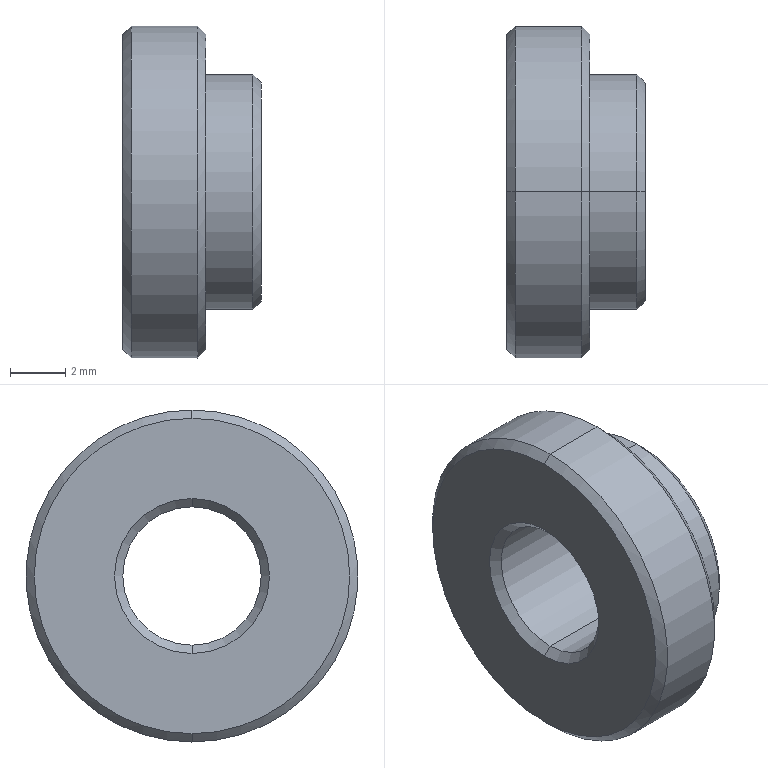Part | STEP file | ftcm_d8_5_h12_v5_0_t3_0_l5_0_2_03 | 1 solid | 19 faces | box 5 x 12 x 12 mm | volume 348.627 mm3 | cone 10 | cylinder 6 | plane 3 | commonest cylinder face diameters 5 x2 8.5 x2 12 x2
STEP:
#1=CARTESIAN_POINT('',(0.,0.,0.));
#2=DIRECTION('',(0.,0.,1.));
#3=DIRECTION('',(1.,0.,0.));
#4=AXIS2_PLACEMENT_3D('',#1,#2,#3);
#5=CARTESIAN_POINT('',(0.,0.,5.7));
#6=VERTEX_POINT('',#5);
#7=CARTESIAN_POINT('',(0.,0.,-5.7));
#8=VERTEX_POINT('',#7);
#9=CARTESIAN_POINT('',(0.,0.,0.));
#10=DIRECTION('',(-1.,0.,0.));
#11=DIRECTION('',(0.,0.,-1.));
#12=AXIS2_PLACEMENT_3D('',#9,#10,#11);
#13=CIRCLE('',#12,5.7);
#14=CARTESIAN_POINT('',(0.3,0.,0.));
#15=DIRECTION('',(1.,0.,0.));
#16=DIRECTION('',(0.,0.,-1.));
#17=AXIS2_PLACEMENT_3D('',#14,#15,#16);
#18=CONICAL_SURFACE('',#17,6.,0.7854);
#19=CARTESIAN_POINT('',(6.283,-0.3));
#20=DIRECTION('',(-1.,0.));
#21=VECTOR('',#20,1.);
#22=LINE('',#19,#21);
#23=(GEOMETRIC_REPRESENTATION_CONTEXT(2)PARAMETRIC_REPRESENTATION_CONTEXT()REPRESENTATION_CONTEXT('',''));
#24=DEFINITIONAL_REPRESENTATION('',(#22),#23);
#25=PCURVE('',#18,#24);
#26=CARTESIAN_POINT('',(0.,4.25,0.));
#27=DIRECTION('',(-1.,0.,0.));
#28=DIRECTION('',(0.,0.,1.));
#29=AXIS2_PLACEMENT_3D('',#26,#27,#28);
#30=PLANE('',#29);
#31=CARTESIAN_POINT('',(0.,-4.25));
#32=DIRECTION('',(-1.,0.));
#33=AXIS2_PLACEMENT_2D('',#31,#32);
#34=CIRCLE('',#33,5.7);
#35=(GEOMETRIC_REPRESENTATION_CONTEXT(2)PARAMETRIC_REPRESENTATION_CONTEXT()REPRESENTATION_CONTEXT('',''));
#36=DEFINITIONAL_REPRESENTATION('',(#34),#35);
#37=PCURVE('',#30,#36);
#38=SURFACE_CURVE('',#13,(#25,#37),.PCURVE_S1.);
#39=EDGE_CURVE('',#6,#8,#38,.T.);
#40=ORIENTED_EDGE('',*,*,#39,.F.);
#41=CARTESIAN_POINT('',(0.3,0.,6.));
#42=VERTEX_POINT('',#41);
#43=CARTESIAN_POINT('',(0.3,0.,6.));
#44=DIRECTION('',(0.7071,0.,0.7071));
#45=VECTOR('',#44,1.);
#46=LINE('',#43,#45);
#47=CARTESIAN_POINT('',(3.142,0.));
#48=DIRECTION('',(0.,1.));
#49=VECTOR('',#48,1.);
#50=LINE('',#47,#49);
#51=(GEOMETRIC_REPRESENTATION_CONTEXT(2)PARAMETRIC_REPRESENTATION_CONTEXT()REPRESENTATION_CONTEXT('',''));
#52=DEFINITIONAL_REPRESENTATION('',(#50),#51);
#53=PCURVE('',#18,#52);
#54=CARTESIAN_POINT('',(0.3,0.,0.));
#55=DIRECTION('',(1.,0.,0.));
#56=DIRECTION('',(0.,0.,-1.));
#57=AXIS2_PLACEMENT_3D('',#54,#55,#56);
#58=CONICAL_SURFACE('',#57,6.,0.7854);
#59=CARTESIAN_POINT('',(3.142,0.));
#60=DIRECTION('',(0.,1.));
#61=VECTOR('',#60,1.);
#62=LINE('',#59,#61);
#63=(GEOMETRIC_REPRESENTATION_CONTEXT(2)PARAMETRIC_REPRESENTATION_CONTEXT()REPRESENTATION_CONTEXT('',''));
#64=DEFINITIONAL_REPRESENTATION('',(#62),#63);
#65=PCURVE('',#58,#64);
#66=SURFACE_CURVE('',#46,(#53,#65),.PCURVE_S1.);
#67=EDGE_CURVE('',#6,#42,#66,.T.);
#68=ORIENTED_EDGE('',*,*,#67,.T.);
#69=CARTESIAN_POINT('',(0.3,0.,-6.));
#70=VERTEX_POINT('',#69);
#71=CARTESIAN_POINT('',(0.3,0.,0.));
#72=DIRECTION('',(-1.,0.,0.));
#73=DIRECTION('',(0.,1.,0.));
#74=AXIS2_PLACEMENT_3D('',#71,#72,#73);
#75=CIRCLE('',#74,6.);
#76=CARTESIAN_POINT('',(7.854,0.));
#77=DIRECTION('',(-1.,0.));
#78=VECTOR('',#77,1.);
#79=LINE('',#76,#78);
#80=(GEOMETRIC_REPRESENTATION_CONTEXT(2)PARAMETRIC_REPRESENTATION_CONTEXT()REPRESENTATION_CONTEXT('',''));
#81=DEFINITIONAL_REPRESENTATION('',(#79),#80);
#82=PCURVE('',#18,#81);
#83=CARTESIAN_POINT('',(1.5,0.,0.));
#84=DIRECTION('',(1.,0.,0.));
#85=DIRECTION('',(0.,0.,-1.));
#86=AXIS2_PLACEMENT_3D('',#83,#84,#85);
#87=CYLINDRICAL_SURFACE('',#86,6.);
#88=CARTESIAN_POINT('',(7.854,-1.2));
#89=DIRECTION('',(-1.,0.));
#90=VECTOR('',#89,1.);
#91=LINE('',#88,#90);
#92=(GEOMETRIC_REPRESENTATION_CONTEXT(2)PARAMETRIC_REPRESENTATION_CONTEXT()REPRESENTATION_CONTEXT('',''));
#93=DEFINITIONAL_REPRESENTATION('',(#91),#92);
#94=PCURVE('',#87,#93);
#95=SURFACE_CURVE('',#75,(#82,#94),.PCURVE_S1.);
#96=EDGE_CURVE('',#42,#70,#95,.T.);
#97=ORIENTED_EDGE('',*,*,#96,.T.);
#98=CARTESIAN_POINT('',(0.3,0.,-6.));
#99=DIRECTION('',(0.7071,0.,-0.7071));
#100=VECTOR('',#99,1.);
#101=LINE('',#98,#100);
#102=CARTESIAN_POINT('',(0.,0.));
#103=DIRECTION('',(0.,1.));
#104=VECTOR('',#103,1.);
#105=LINE('',#102,#104);
#106=(GEOMETRIC_REPRESENTATION_CONTEXT(2)PARAMETRIC_REPRESENTATION_CONTEXT()REPRESENTATION_CONTEXT('',''));
#107=DEFINITIONAL_REPRESENTATION('',(#105),#106);
#108=PCURVE('',#18,#107);
#109=CARTESIAN_POINT('',(6.283,0.));
#110=DIRECTION('',(0.,1.));
#111=VECTOR('',#110,1.);
#112=LINE('',#109,#111);
#113=(GEOMETRIC_REPRESENTATION_CONTEXT(2)PARAMETRIC_REPRESENTATION_CONTEXT()REPRESENTATION_CONTEXT('',''));
#114=DEFINITIONAL_REPRESENTATION('',(#112),#113);
#115=PCURVE('',#58,#114);
#116=SURFACE_CURVE('',#101,(#108,#115),.PCURVE_S1.);
#117=EDGE_CURVE('',#8,#70,#116,.T.);
#118=ORIENTED_EDGE('',*,*,#117,.F.);
#119=EDGE_LOOP('',(#40,#68,#97,#118));
#120=FACE_BOUND('',#119,.T.);
#121=ADVANCED_FACE('',(#120),#18,.T.);
#122=CARTESIAN_POINT('',(0.3,0.,2.5));
#123=VERTEX_POINT('',#122);
#124=CARTESIAN_POINT('',(0.,0.,2.8));
#125=VERTEX_POINT('',#124);
#126=CARTESIAN_POINT('',(0.,0.,2.8));
#127=DIRECTION('',(-0.7071,0.,0.7071));
#128=VECTOR('',#127,1.);
#129=LINE('',#126,#128);
#130=CARTESIAN_POINT('',(0.,0.,0.));
#131=DIRECTION('',(-1.,0.,0.));
#132=DIRECTION('',(0.,0.,1.));
#133=AXIS2_PLACEMENT_3D('',#130,#131,#132);
#134=CONICAL_SURFACE('',#133,2.8,0.7854);
#135=CARTESIAN_POINT('',(6.283,0.));
#136=DIRECTION('',(0.,1.));
#137=VECTOR('',#136,1.);
#138=LINE('',#135,#137);
#139=(GEOMETRIC_REPRESENTATION_CONTEXT(2)PARAMETRIC_REPRESENTATION_CONTEXT()REPRESENTATION_CONTEXT('',''));
#140=DEFINITIONAL_REPRESENTATION('',(#138),#139);
#141=PCURVE('',#134,#140);
#142=CARTESIAN_POINT('',(0.,0.,0.));
#143=DIRECTION('',(-1.,0.,0.));
#144=DIRECTION('',(0.,0.,1.));
#145=AXIS2_PLACEMENT_3D('',#142,#143,#144);
#146=CONICAL_SURFACE('',#145,2.8,0.7854);
#147=CARTESIAN_POINT('',(0.,0.));
#148=DIRECTION('',(0.,1.));
#149=VECTOR('',#148,1.);
#150=LINE('',#147,#149);
#151=(GEOMETRIC_REPRESENTATION_CONTEXT(2)PARAMETRIC_REPRESENTATION_CONTEXT()REPRESENTATION_CONTEXT('',''));
#152=DEFINITIONAL_REPRESENTATION('',(#150),#151);
#153=PCURVE('',#146,#152);
#154=SURFACE_CURVE('',#129,(#141,#153),.PCURVE_S1.);
#155=EDGE_CURVE('',#123,#125,#154,.T.);
#156=ORIENTED_EDGE('',*,*,#155,.T.);
#157=CARTESIAN_POINT('',(0.,0.,-2.8));
#158=VERTEX_POINT('',#157);
#159=CARTESIAN_POINT('',(0.,0.,0.));
#160=DIRECTION('',(1.,0.,0.));
#161=DIRECTION('',(0.,0.,1.));
#162=AXIS2_PLACEMENT_3D('',#159,#160,#161);
#163=CIRCLE('',#162,2.8);
#164=CARTESIAN_POINT('',(6.283,0.));
#165=DIRECTION('',(-1.,0.));
#166=VECTOR('',#165,1.);
#167=LINE('',#164,#166);
#168=(GEOMETRIC_REPRESENTATION_CONTEXT(2)PARAMETRIC_REPRESENTATION_CONTEXT()REPRESENTATION_CONTEXT('',''));
#169=DEFINITIONAL_REPRESENTATION('',(#167),#168);
#170=PCURVE('',#134,#169);
#171=CARTESIAN_POINT('',(2.8,-4.25));
#172=CARTESIAN_POINT('',(2.8,-9.1));
#173=CARTESIAN_POINT('',(-1.4,-6.675));
#174=CARTESIAN_POINT('',(-5.6,-4.25));
#175=CARTESIAN_POINT('',(-1.4,-1.825));
#176=CARTESIAN_POINT('',(2.8,0.5997));
#177=CARTESIAN_POINT('',(2.8,-4.25));
#178=(BOUNDED_CURVE()B_SPLINE_CURVE(2,(#171,#172,#173,#174,#175,#176,#177),.UNSPECIFIED.,.T.,.F.)B_SPLINE_CURVE_WITH_KNOTS((1,2,2,2,2,1),(-2.094,0.,2.094,4.189,6.283,8.378),.UNSPECIFIED.)CURVE()GEOMETRIC_REPRESENTATION_ITEM()RATIONAL_B_SPLINE_CURVE((1.,0.5,1.,0.5,1.,0.5,1.))REPRESENTATION_ITEM(''));
#179=(GEOMETRIC_REPRESENTATION_CONTEXT(2)PARAMETRIC_REPRESENTATION_CONTEXT()REPRESENTATION_CONTEXT('',''));
#180=DEFINITIONAL_REPRESENTATION('',(#178),#179);
#181=PCURVE('',#30,#180);
#182=SURFACE_CURVE('',#163,(#170,#181),.PCURVE_S1.);
#183=EDGE_CURVE('',#125,#158,#182,.T.);
#184=ORIENTED_EDGE('',*,*,#183,.T.);
#185=CARTESIAN_POINT('',(0.3,0.,-2.5));
#186=VERTEX_POINT('',#185);
#187=CARTESIAN_POINT('',(0.,0.,-2.8));
#188=DIRECTION('',(-0.7071,0.,-0.7071));
#189=VECTOR('',#188,1.);
#190=LINE('',#187,#189);
#191=CARTESIAN_POINT('',(3.142,0.));
#192=DIRECTION('',(0.,1.));
#193=VECTOR('',#192,1.);
#194=LINE('',#191,#193);
#195=(GEOMETRIC_REPRESENTATION_CONTEXT(2)PARAMETRIC_REPRESENTATION_CONTEXT()REPRESENTATION_CONTEXT('',''));
#196=DEFINITIONAL_REPRESENTATION('',(#194),#195);
#197=PCURVE('',#134,#196);
#198=CARTESIAN_POINT('',(3.142,0.));
#199=DIRECTION('',(0.,1.));
#200=VECTOR('',#199,1.);
#201=LINE('',#198,#200);
#202=(GEOMETRIC_REPRESENTATION_CONTEXT(2)PARAMETRIC_REPRESENTATION_CONTEXT()REPRESENTATION_CONTEXT('',''));
#203=DEFINITIONAL_REPRESENTATION('',(#201),#202);
#204=PCURVE('',#146,#203);
#205=SURFACE_CURVE('',#190,(#197,#204),.PCURVE_S1.);
#206=EDGE_CURVE('',#186,#158,#205,.T.);
#207=ORIENTED_EDGE('',*,*,#206,.F.);
#208=CARTESIAN_POINT('',(0.3,0.,0.));
#209=DIRECTION('',(-1.,0.,0.));
#210=DIRECTION('',(0.,1.,0.));
#211=AXIS2_PLACEMENT_3D('',#208,#209,#210);
#212=CIRCLE('',#211,2.5);
#213=CARTESIAN_POINT('',(1.571,-0.3));
#214=DIRECTION('',(1.,0.));
#215=VECTOR('',#214,1.);
#216=LINE('',#213,#215);
#217=(GEOMETRIC_REPRESENTATION_CONTEXT(2)PARAMETRIC_REPRESENTATION_CONTEXT()REPRESENTATION_CONTEXT('',''));
#218=DEFINITIONAL_REPRESENTATION('',(#216),#217);
#219=PCURVE('',#134,#218);
#220=CARTESIAN_POINT('',(2.5,0.,0.));
#221=DIRECTION('',(1.,0.,0.));
#222=DIRECTION('',(0.,0.,-1.));
#223=AXIS2_PLACEMENT_3D('',#220,#221,#222);
#224=CYLINDRICAL_SURFACE('',#223,2.5);
#225=CARTESIAN_POINT('',(7.854,-2.2));
#226=DIRECTION('',(-1.,0.));
#227=VECTOR('',#226,1.);
#228=LINE('',#225,#227);
#229=(GEOMETRIC_REPRESENTATION_CONTEXT(2)PARAMETRIC_REPRESENTATION_CONTEXT()REPRESENTATION_CONTEXT('',''));
#230=DEFINITIONAL_REPRESENTATION('',(#228),#229);
#231=PCURVE('',#224,#230);
#232=SURFACE_CURVE('',#212,(#219,#231),.PCURVE_S1.);
#233=EDGE_CURVE('',#186,#123,#232,.T.);
#234=ORIENTED_EDGE('',*,*,#233,.T.);
#235=EDGE_LOOP('',(#156,#184,#207,#234));
#236=FACE_BOUND('',#235,.F.);
#237=ADVANCED_FACE('',(#236),#134,.F.);
#238=ORIENTED_EDGE('',*,*,#96,.F.);
#239=CARTESIAN_POINT('',(2.7,0.,6.));
#240=VERTEX_POINT('',#239);
#241=CARTESIAN_POINT('',(1.5,0.,6.));
#242=DIRECTION('',(1.,0.,0.));
#243=VECTOR('',#242,1.);
#244=LINE('',#241,#243);
#245=CARTESIAN_POINT('',(3.142,0.));
#246=DIRECTION('',(0.,1.));
#247=VECTOR('',#246,1.);
#248=LINE('',#245,#247);
#249=(GEOMETRIC_REPRESENTATION_CONTEXT(2)PARAMETRIC_REPRESENTATION_CONTEXT()REPRESENTATION_CONTEXT('',''));
#250=DEFINITIONAL_REPRESENTATION('',(#248),#249);
#251=PCURVE('',#87,#250);
#252=CARTESIAN_POINT('',(1.5,0.,0.));
#253=DIRECTION('',(1.,0.,0.));
#254=DIRECTION('',(0.,0.,-1.));
#255=AXIS2_PLACEMENT_3D('',#252,#253,#254);
#256=CYLINDRICAL_SURFACE('',#255,6.);
#257=CARTESIAN_POINT('',(3.142,0.));
#258=DIRECTION('',(0.,1.));
#259=VECTOR('',#258,1.);
#260=LINE('',#257,#259);
#261=(GEOMETRIC_REPRESENTATION_CONTEXT(2)PARAMETRIC_REPRESENTATION_CONTEXT()REPRESENTATION_CONTEXT('',''));
#262=DEFINITIONAL_REPRESENTATION('',(#260),#261);
#263=PCURVE('',#256,#262);
#264=SURFACE_CURVE('',#244,(#251,#263),.PCURVE_S1.);
#265=EDGE_CURVE('',#42,#240,#264,.T.);
#266=ORIENTED_EDGE('',*,*,#265,.T.);
#267=CARTESIAN_POINT('',(2.7,0.,-6.));
#268=VERTEX_POINT('',#267);
#269=CARTESIAN_POINT('',(2.7,0.,0.));
#270=DIRECTION('',(-1.,0.,0.));
#271=DIRECTION('',(0.,0.,-1.));
#272=AXIS2_PLACEMENT_3D('',#269,#270,#271);
#273=CIRCLE('',#272,6.);
#274=CARTESIAN_POINT('',(6.283,1.2));
#275=DIRECTION('',(-1.,0.));
#276=VECTOR('',#275,1.);
#277=LINE('',#274,#276);
#278=(GEOMETRIC_REPRESENTATION_CONTEXT(2)PARAMETRIC_REPRESENTATION_CONTEXT()REPRESENTATION_CONTEXT('',''));
#279=DEFINITIONAL_REPRESENTATION('',(#277),#278);
#280=PCURVE('',#87,#279);
#281=CARTESIAN_POINT('',(2.7,0.,0.));
#282=DIRECTION('',(-1.,0.,0.));
#283=DIRECTION('',(0.,0.,1.));
#284=AXIS2_PLACEMENT_3D('',#281,#282,#283);
#285=CONICAL_SURFACE('',#284,6.,0.7854);
#286=CARTESIAN_POINT('',(-3.142,0.));
#287=DIRECTION('',(1.,0.));
#288=VECTOR('',#287,1.);
#289=LINE('',#286,#288);
#290=(GEOMETRIC_REPRESENTATION_CONTEXT(2)PARAMETRIC_REPRESENTATION_CONTEXT()REPRESENTATION_CONTEXT('',''));
#291=DEFINITIONAL_REPRESENTATION('',(#289),#290);
#292=PCURVE('',#285,#291);
#293=SURFACE_CURVE('',#273,(#280,#292),.PCURVE_S1.);
#294=EDGE_CURVE('',#240,#268,#293,.T.);
#295=ORIENTED_EDGE('',*,*,#294,.T.);
#296=CARTESIAN_POINT('',(1.5,0.,-6.));
#297=DIRECTION('',(1.,0.,0.));
#298=VECTOR('',#297,1.);
#299=LINE('',#296,#298);
#300=CARTESIAN_POINT('',(0.,0.));
#301=DIRECTION('',(0.,1.));
#302=VECTOR('',#301,1.);
#303=LINE('',#300,#302);
#304=(GEOMETRIC_REPRESENTATION_CONTEXT(2)PARAMETRIC_REPRESENTATION_CONTEXT()REPRESENTATION_CONTEXT('',''));
#305=DEFINITIONAL_REPRESENTATION('',(#303),#304);
#306=PCURVE('',#87,#305);
#307=CARTESIAN_POINT('',(6.283,0.));
#308=DIRECTION('',(0.,1.));
#309=VECTOR('',#308,1.);
#310=LINE('',#307,#309);
#311=(GEOMETRIC_REPRESENTATION_CONTEXT(2)PARAMETRIC_REPRESENTATION_CONTEXT()REPRESENTATION_CONTEXT('',''));
#312=DEFINITIONAL_REPRESENTATION('',(#310),#311);
#313=PCURVE('',#256,#312);
#314=SURFACE_CURVE('',#299,(#306,#313),.PCURVE_S1.);
#315=EDGE_CURVE('',#70,#268,#314,.T.);
#316=ORIENTED_EDGE('',*,*,#315,.F.);
#317=EDGE_LOOP('',(#238,#266,#295,#316));
#318=FACE_BOUND('',#317,.T.);
#319=ADVANCED_FACE('',(#318),#87,.T.);
#320=CARTESIAN_POINT('',(4.7,0.,-2.5));
#321=VERTEX_POINT('',#320);
#322=CARTESIAN_POINT('',(2.5,0.,-2.5));
#323=DIRECTION('',(1.,0.,0.));
#324=VECTOR('',#323,1.);
#325=LINE('',#322,#324);
#326=CARTESIAN_POINT('',(6.283,0.));
#327=DIRECTION('',(0.,1.));
#328=VECTOR('',#327,1.);
#329=LINE('',#326,#328);
#330=(GEOMETRIC_REPRESENTATION_CONTEXT(2)PARAMETRIC_REPRESENTATION_CONTEXT()REPRESENTATION_CONTEXT('',''));
#331=DEFINITIONAL_REPRESENTATION('',(#329),#330);
#332=PCURVE('',#224,#331);
#333=CARTESIAN_POINT('',(2.5,0.,0.));
#334=DIRECTION('',(1.,0.,0.));
#335=DIRECTION('',(0.,0.,-1.));
#336=AXIS2_PLACEMENT_3D('',#333,#334,#335);
#337=CYLINDRICAL_SURFACE('',#336,2.5);
#338=CARTESIAN_POINT('',(0.,0.));
#339=DIRECTION('',(0.,1.));
#340=VECTOR('',#339,1.);
#341=LINE('',#338,#340);
#342=(GEOMETRIC_REPRESENTATION_CONTEXT(2)PARAMETRIC_REPRESENTATION_CONTEXT()REPRESENTATION_CONTEXT('',''));
#343=DEFINITIONAL_REPRESENTATION('',(#341),#342);
#344=PCURVE('',#337,#343);
#345=SURFACE_CURVE('',#325,(#332,#344),.PCURVE_S1.);
#346=EDGE_CURVE('',#186,#321,#345,.T.);
#347=ORIENTED_EDGE('',*,*,#346,.T.);
#348=CARTESIAN_POINT('',(4.7,0.,2.5));
#349=VERTEX_POINT('',#348);
#350=CARTESIAN_POINT('',(4.7,0.,0.));
#351=DIRECTION('',(-1.,0.,0.));
#352=DIRECTION('',(0.,0.,-1.));
#353=AXIS2_PLACEMENT_3D('',#350,#351,#352);
#354=CIRCLE('',#353,2.5);
#355=CARTESIAN_POINT('',(6.283,2.2));
#356=DIRECTION('',(-1.,0.));
#357=VECTOR('',#356,1.);
#358=LINE('',#355,#357);
#359=(GEOMETRIC_REPRESENTATION_CONTEXT(2)PARAMETRIC_REPRESENTATION_CONTEXT()REPRESENTATION_CONTEXT('',''));
#360=DEFINITIONAL_REPRESENTATION('',(#358),#359);
#361=PCURVE('',#224,#360);
#362=CARTESIAN_POINT('',(5.,0.,0.));
#363=DIRECTION('',(1.,0.,0.));
#364=DIRECTION('',(0.,0.,-1.));
#365=AXIS2_PLACEMENT_3D('',#362,#363,#364);
#366=CONICAL_SURFACE('',#365,2.8,0.7854);
#367=CARTESIAN_POINT('',(6.283,-0.3));
#368=DIRECTION('',(-1.,0.));
#369=VECTOR('',#368,1.);
#370=LINE('',#367,#369);
#371=(GEOMETRIC_REPRESENTATION_CONTEXT(2)PARAMETRIC_REPRESENTATION_CONTEXT()REPRESENTATION_CONTEXT('',''));
#372=DEFINITIONAL_REPRESENTATION('',(#370),#371);
#373=PCURVE('',#366,#372);
#374=SURFACE_CURVE('',#354,(#361,#373),.PCURVE_S1.);
#375=EDGE_CURVE('',#321,#349,#374,.T.);
#376=ORIENTED_EDGE('',*,*,#375,.T.);
#377=CARTESIAN_POINT('',(2.5,0.,2.5));
#378=DIRECTION('',(1.,0.,0.));
#379=VECTOR('',#378,1.);
#380=LINE('',#377,#379);
#381=CARTESIAN_POINT('',(3.142,0.));
#382=DIRECTION('',(0.,1.));
#383=VECTOR('',#382,1.);
#384=LINE('',#381,#383);
#385=(GEOMETRIC_REPRESENTATION_CONTEXT(2)PARAMETRIC_REPRESENTATION_CONTEXT()REPRESENTATION_CONTEXT('',''));
#386=DEFINITIONAL_REPRESENTATION('',(#384),#385);
#387=PCURVE('',#224,#386);
#388=CARTESIAN_POINT('',(3.142,0.));
#389=DIRECTION('',(0.,1.));
#390=VECTOR('',#389,1.);
#391=LINE('',#388,#390);
#392=(GEOMETRIC_REPRESENTATION_CONTEXT(2)PARAMETRIC_REPRESENTATION_CONTEXT()REPRESENTATION_CONTEXT('',''));
#393=DEFINITIONAL_REPRESENTATION('',(#391),#392);
#394=PCURVE('',#337,#393);
#395=SURFACE_CURVE('',#380,(#387,#394),.PCURVE_S1.);
#396=EDGE_CURVE('',#123,#349,#395,.T.);
#397=ORIENTED_EDGE('',*,*,#396,.F.);
#398=ORIENTED_EDGE('',*,*,#233,.F.);
#399=EDGE_LOOP('',(#347,#376,#397,#398));
#400=FACE_BOUND('',#399,.F.);
#401=ADVANCED_FACE('',(#400),#224,.F.);
#402=CARTESIAN_POINT('',(3.,0.,5.7));
#403=VERTEX_POINT('',#402);
#404=CARTESIAN_POINT('',(3.,0.,-5.7));
#405=VERTEX_POINT('',#404);
#406=CARTESIAN_POINT('',(3.,0.,0.));
#407=DIRECTION('',(-1.,0.,0.));
#408=DIRECTION('',(0.,0.,1.));
#409=AXIS2_PLACEMENT_3D('',#406,#407,#408);
#410=CIRCLE('',#409,5.7);
#411=CARTESIAN_POINT('',(0.,-0.3));
#412=DIRECTION('',(1.,0.));
#413=VECTOR('',#412,1.);
#414=LINE('',#411,#413);
#415=(GEOMETRIC_REPRESENTATION_CONTEXT(2)PARAMETRIC_REPRESENTATION_CONTEXT()REPRESENTATION_CONTEXT('',''));
#416=DEFINITIONAL_REPRESENTATION('',(#414),#415);
#417=PCURVE('',#285,#416);
#418=CARTESIAN_POINT('',(3.,4.975,0.));
#419=DIRECTION('',(1.,0.,0.));
#420=DIRECTION('',(0.,0.,-1.));
#421=AXIS2_PLACEMENT_3D('',#418,#419,#420);
#422=PLANE('',#421);
#423=CARTESIAN_POINT('',(-5.7,-4.975));
#424=CARTESIAN_POINT('',(-5.7,4.898));
#425=CARTESIAN_POINT('',(2.85,-0.03866));
#426=CARTESIAN_POINT('',(11.4,-4.975));
#427=CARTESIAN_POINT('',(2.85,-9.911));
#428=CARTESIAN_POINT('',(-5.7,-14.848));
#429=CARTESIAN_POINT('',(-5.7,-4.975));
#430=(BOUNDED_CURVE()B_SPLINE_CURVE(2,(#423,#424,#425,#426,#427,#428,#429),.UNSPECIFIED.,.T.,.F.)B_SPLINE_CURVE_WITH_KNOTS((1,2,2,2,2,1),(-2.094,0.,2.094,4.189,6.283,8.378),.UNSPECIFIED.)CURVE()GEOMETRIC_REPRESENTATION_ITEM()RATIONAL_B_SPLINE_CURVE((1.,0.5,1.,0.5,1.,0.5,1.))REPRESENTATION_ITEM(''));
#431=(GEOMETRIC_REPRESENTATION_CONTEXT(2)PARAMETRIC_REPRESENTATION_CONTEXT()REPRESENTATION_CONTEXT('',''));
#432=DEFINITIONAL_REPRESENTATION('',(#430),#431);
#433=PCURVE('',#422,#432);
#434=SURFACE_CURVE('',#410,(#417,#433),.PCURVE_S1.);
#435=EDGE_CURVE('',#403,#405,#434,.T.);
#436=ORIENTED_EDGE('',*,*,#435,.T.);
#437=CARTESIAN_POINT('',(2.7,0.,-6.));
#438=DIRECTION('',(-0.7071,0.,-0.7071));
#439=VECTOR('',#438,1.);
#440=LINE('',#437,#439);
#441=CARTESIAN_POINT('',(3.142,0.));
#442=DIRECTION('',(0.,1.));
#443=VECTOR('',#442,1.);
#444=LINE('',#441,#443);
#445=(GEOMETRIC_REPRESENTATION_CONTEXT(2)PARAMETRIC_REPRESENTATION_CONTEXT()REPRESENTATION_CONTEXT('',''));
#446=DEFINITIONAL_REPRESENTATION('',(#444),#445);
#447=PCURVE('',#285,#446);
#448=CARTESIAN_POINT('',(2.7,0.,0.));
#449=DIRECTION('',(-1.,0.,0.));
#450=DIRECTION('',(0.,0.,1.));
#451=AXIS2_PLACEMENT_3D('',#448,#449,#450);
#452=CONICAL_SURFACE('',#451,6.,0.7854);
#453=CARTESIAN_POINT('',(3.142,0.));
#454=DIRECTION('',(0.,1.));
#455=VECTOR('',#454,1.);
#456=LINE('',#453,#455);
#457=(GEOMETRIC_REPRESENTATION_CONTEXT(2)PARAMETRIC_REPRESENTATION_CONTEXT()REPRESENTATION_CONTEXT('',''));
#458=DEFINITIONAL_REPRESENTATION('',(#456),#457);
#459=PCURVE('',#452,#458);
#460=SURFACE_CURVE('',#440,(#447,#459),.PCURVE_S1.);
#461=EDGE_CURVE('',#405,#268,#460,.T.);
#462=ORIENTED_EDGE('',*,*,#461,.T.);
#463=ORIENTED_EDGE('',*,*,#294,.F.);
#464=CARTESIAN_POINT('',(2.7,0.,6.));
#465=DIRECTION('',(-0.7071,0.,0.7071));
#466=VECTOR('',#465,1.);
#467=LINE('',#464,#466);
#468=CARTESIAN_POINT('',(0.,0.));
#469=DIRECTION('',(0.,1.));
#470=VECTOR('',#469,1.);
#471=LINE('',#468,#470);
#472=(GEOMETRIC_REPRESENTATION_CONTEXT(2)PARAMETRIC_REPRESENTATION_CONTEXT()REPRESENTATION_CONTEXT('',''));
#473=DEFINITIONAL_REPRESENTATION('',(#471),#472);
#474=PCURVE('',#285,#473);
#475=CARTESIAN_POINT('',(6.283,0.));
#476=DIRECTION('',(0.,1.));
#477=VECTOR('',#476,1.);
#478=LINE('',#475,#477);
#479=(GEOMETRIC_REPRESENTATION_CONTEXT(2)PARAMETRIC_REPRESENTATION_CONTEXT()REPRESENTATION_CONTEXT('',''));
#480=DEFINITIONAL_REPRESENTATION('',(#478),#479);
#481=PCURVE('',#452,#480);
#482=SURFACE_CURVE('',#467,(#474,#481),.PCURVE_S1.);
#483=EDGE_CURVE('',#403,#240,#482,.T.);
#484=ORIENTED_EDGE('',*,*,#483,.F.);
#485=EDGE_LOOP('',(#436,#462,#463,#484));
#486=FACE_BOUND('',#485,.T.);
#487=ADVANCED_FACE('',(#486),#285,.T.);
#488=CARTESIAN_POINT('',(5.,0.,-2.8));
#489=VERTEX_POINT('',#488);
#490=CARTESIAN_POINT('',(5.,0.,-2.8));
#491=DIRECTION('',(0.7071,0.,-0.7071));
#492=VECTOR('',#491,1.);
#493=LINE('',#490,#492);
#494=CARTESIAN_POINT('',(6.283,0.));
#495=DIRECTION('',(0.,1.));
#496=VECTOR('',#495,1.);
#497=LINE('',#494,#496);
#498=(GEOMETRIC_REPRESENTATION_CONTEXT(2)PARAMETRIC_REPRESENTATION_CONTEXT()REPRESENTATION_CONTEXT('',''));
#499=DEFINITIONAL_REPRESENTATION('',(#497),#498);
#500=PCURVE('',#366,#499);
#501=CARTESIAN_POINT('',(5.,0.,0.));
#502=DIRECTION('',(1.,0.,0.));
#503=DIRECTION('',(0.,0.,-1.));
#504=AXIS2_PLACEMENT_3D('',#501,#502,#503);
#505=CONICAL_SURFACE('',#504,2.8,0.7854);
#506=CARTESIAN_POINT('',(0.,0.));
#507=DIRECTION('',(0.,1.));
#508=VECTOR('',#507,1.);
#509=LINE('',#506,#508);
#510=(GEOMETRIC_REPRESENTATION_CONTEXT(2)PARAMETRIC_REPRESENTATION_CONTEXT()REPRESENTATION_CONTEXT('',''));
#511=DEFINITIONAL_REPRESENTATION('',(#509),#510);
#512=PCURVE('',#505,#511);
#513=SURFACE_CURVE('',#493,(#500,#512),.PCURVE_S1.);
#514=EDGE_CURVE('',#321,#489,#513,.T.);
#515=ORIENTED_EDGE('',*,*,#514,.T.);
#516=CARTESIAN_POINT('',(5.,0.,2.8));
#517=VERTEX_POINT('',#516);
#518=CARTESIAN_POINT('',(5.,0.,0.));
#519=DIRECTION('',(-1.,0.,0.));
#520=DIRECTION('',(0.,0.,-1.));
#521=AXIS2_PLACEMENT_3D('',#518,#519,#520);
#522=CIRCLE('',#521,2.8);
#523=CARTESIAN_POINT('',(6.283,0.));
#524=DIRECTION('',(-1.,0.));
#525=VECTOR('',#524,1.);
#526=LINE('',#523,#525);
#527=(GEOMETRIC_REPRESENTATION_CONTEXT(2)PARAMETRIC_REPRESENTATION_CONTEXT()REPRESENTATION_CONTEXT('',''));
#528=DEFINITIONAL_REPRESENTATION('',(#526),#527);
#529=PCURVE('',#366,#528);
#530=CARTESIAN_POINT('',(5.,3.375,0.));
#531=DIRECTION('',(1.,0.,0.));
#532=DIRECTION('',(0.,0.,-1.));
#533=AXIS2_PLACEMENT_3D('',#530,#531,#532);
#534=PLANE('',#533);
#535=CARTESIAN_POINT('',(2.8,-3.375));
#536=CARTESIAN_POINT('',(2.8,-8.225));
#537=CARTESIAN_POINT('',(-1.4,-5.8));
#538=CARTESIAN_POINT('',(-5.6,-3.375));
#539=CARTESIAN_POINT('',(-1.4,-0.9501));
#540=CARTESIAN_POINT('',(2.8,1.475));
#541=CARTESIAN_POINT('',(2.8,-3.375));
#542=(BOUNDED_CURVE()B_SPLINE_CURVE(2,(#535,#536,#537,#538,#539,#540,#541),.UNSPECIFIED.,.T.,.F.)B_SPLINE_CURVE_WITH_KNOTS((1,2,2,2,2,1),(-2.094,0.,2.094,4.189,6.283,8.378),.UNSPECIFIED.)CURVE()GEOMETRIC_REPRESENTATION_ITEM()RATIONAL_B_SPLINE_CURVE((1.,0.5,1.,0.5,1.,0.5,1.))REPRESENTATION_ITEM(''));
#543=(GEOMETRIC_REPRESENTATION_CONTEXT(2)PARAMETRIC_REPRESENTATION_CONTEXT()REPRESENTATION_CONTEXT('',''));
#544=DEFINITIONAL_REPRESENTATION('',(#542),#543);
#545=PCURVE('',#534,#544);
#546=SURFACE_CURVE('',#522,(#529,#545),.PCURVE_S1.);
#547=EDGE_CURVE('',#489,#517,#546,.T.);
#548=ORIENTED_EDGE('',*,*,#547,.T.);
#549=CARTESIAN_POINT('',(5.,0.,2.8));
#550=DIRECTION('',(0.7071,0.,0.7071));
#551=VECTOR('',#550,1.);
#552=LINE('',#549,#551);
#553=CARTESIAN_POINT('',(3.142,0.));
#554=DIRECTION('',(0.,1.));
#555=VECTOR('',#554,1.);
#556=LINE('',#553,#555);
#557=(GEOMETRIC_REPRESENTATION_CONTEXT(2)PARAMETRIC_REPRESENTATION_CONTEXT()REPRESENTATION_CONTEXT('',''));
#558=DEFINITIONAL_REPRESENTATION('',(#556),#557);
#559=PCURVE('',#366,#558);
#560=CARTESIAN_POINT('',(3.142,0.));
#561=DIRECTION('',(0.,1.));
#562=VECTOR('',#561,1.);
#563=LINE('',#560,#562);
#564=(GEOMETRIC_REPRESENTATION_CONTEXT(2)PARAMETRIC_REPRESENTATION_CONTEXT()REPRESENTATION_CONTEXT('',''));
#565=DEFINITIONAL_REPRESENTATION('',(#563),#564);
#566=PCURVE('',#505,#565);
#567=SURFACE_CURVE('',#552,(#559,#566),.PCURVE_S1.);
#568=EDGE_CURVE('',#349,#517,#567,.T.);
#569=ORIENTED_EDGE('',*,*,#568,.F.);
#570=ORIENTED_EDGE('',*,*,#375,.F.);
#571=EDGE_LOOP('',(#515,#548,#569,#570));
#572=FACE_BOUND('',#571,.F.);
#573=ADVANCED_FACE('',(#572),#366,.F.);
#574=CARTESIAN_POINT('',(3.,0.,4.25));
#575=VERTEX_POINT('',#574);
#576=CARTESIAN_POINT('',(3.,0.,-4.25));
#577=VERTEX_POINT('',#576);
#578=CARTESIAN_POINT('',(3.,0.,0.));
#579=DIRECTION('',(-1.,0.,0.));
#580=DIRECTION('',(0.,0.,-1.));
#581=AXIS2_PLACEMENT_3D('',#578,#579,#580);
#582=CIRCLE('',#581,4.25);
#583=CARTESIAN_POINT('',(3.85,0.,0.));
#584=DIRECTION('',(1.,0.,0.));
#585=DIRECTION('',(0.,0.,-1.));
#586=AXIS2_PLACEMENT_3D('',#583,#584,#585);
#587=CYLINDRICAL_SURFACE('',#586,4.25);
#588=CARTESIAN_POINT('',(6.283,-0.85));
#589=DIRECTION('',(-1.,0.));
#590=VECTOR('',#589,1.);
#591=LINE('',#588,#590);
#592=(GEOMETRIC_REPRESENTATION_CONTEXT(2)PARAMETRIC_REPRESENTATION_CONTEXT()REPRESENTATION_CONTEXT('',''));
#593=DEFINITIONAL_REPRESENTATION('',(#591),#592);
#594=PCURVE('',#587,#593);
#595=CARTESIAN_POINT('',(4.25,-4.975));
#596=CARTESIAN_POINT('',(4.25,-12.336));
#597=CARTESIAN_POINT('',(-2.125,-8.656));
#598=CARTESIAN_POINT('',(-8.5,-4.975));
#599=CARTESIAN_POINT('',(-2.125,-1.294));
#600=CARTESIAN_POINT('',(4.25,2.386));
#601=CARTESIAN_POINT('',(4.25,-4.975));
#602=(BOUNDED_CURVE()B_SPLINE_CURVE(2,(#595,#596,#597,#598,#599,#600,#601),.UNSPECIFIED.,.T.,.F.)B_SPLINE_CURVE_WITH_KNOTS((1,2,2,2,2,1),(-2.094,0.,2.094,4.189,6.283,8.378),.UNSPECIFIED.)CURVE()GEOMETRIC_REPRESENTATION_ITEM()RATIONAL_B_SPLINE_CURVE((1.,0.5,1.,0.5,1.,0.5,1.))REPRESENTATION_ITEM(''));
#603=(GEOMETRIC_REPRESENTATION_CONTEXT(2)PARAMETRIC_REPRESENTATION_CONTEXT()REPRESENTATION_CONTEXT('',''));
#604=DEFINITIONAL_REPRESENTATION('',(#602),#603);
#605=PCURVE('',#422,#604);
#606=SURFACE_CURVE('',#582,(#594,#605),.PCURVE_S1.);
#607=EDGE_CURVE('',#575,#577,#606,.T.);
#608=ORIENTED_EDGE('',*,*,#607,.F.);
#609=CARTESIAN_POINT('',(4.7,0.,4.25));
#610=VERTEX_POINT('',#609);
#611=CARTESIAN_POINT('',(3.85,0.,4.25));
#612=DIRECTION('',(1.,0.,0.));
#613=VECTOR('',#612,1.);
#614=LINE('',#611,#613);
#615=CARTESIAN_POINT('',(3.142,0.));
#616=DIRECTION('',(0.,1.));
#617=VECTOR('',#616,1.);
#618=LINE('',#615,#617);
#619=(GEOMETRIC_REPRESENTATION_CONTEXT(2)PARAMETRIC_REPRESENTATION_CONTEXT()REPRESENTATION_CONTEXT('',''));
#620=DEFINITIONAL_REPRESENTATION('',(#618),#619);
#621=PCURVE('',#587,#620);
#622=CARTESIAN_POINT('',(3.85,0.,0.));
#623=DIRECTION('',(1.,0.,0.));
#624=DIRECTION('',(0.,0.,-1.));
#625=AXIS2_PLACEMENT_3D('',#622,#623,#624);
#626=CYLINDRICAL_SURFACE('',#625,4.25);
#627=CARTESIAN_POINT('',(3.142,0.));
#628=DIRECTION('',(0.,1.));
#629=VECTOR('',#628,1.);
#630=LINE('',#627,#629);
#631=(GEOMETRIC_REPRESENTATION_CONTEXT(2)PARAMETRIC_REPRESENTATION_CONTEXT()REPRESENTATION_CONTEXT('',''));
#632=DEFINITIONAL_REPRESENTATION('',(#630),#631);
#633=PCURVE('',#626,#632);
#634=SURFACE_CURVE('',#614,(#621,#633),.PCURVE_S1.);
#635=EDGE_CURVE('',#575,#610,#634,.T.);
#636=ORIENTED_EDGE('',*,*,#635,.T.);
#637=CARTESIAN_POINT('',(4.7,0.,-4.25));
#638=VERTEX_POINT('',#637);
#639=CARTESIAN_POINT('',(4.7,0.,0.));
#640=DIRECTION('',(-1.,0.,0.));
#641=DIRECTION('',(0.,0.,-1.));
#642=AXIS2_PLACEMENT_3D('',#639,#640,#641);
#643=CIRCLE('',#642,4.25);
#644=CARTESIAN_POINT('',(6.283,0.85));
#645=DIRECTION('',(-1.,0.));
#646=VECTOR('',#645,1.);
#647=LINE('',#644,#646);
#648=(GEOMETRIC_REPRESENTATION_CONTEXT(2)PARAMETRIC_REPRESENTATION_CONTEXT()REPRESENTATION_CONTEXT('',''));
#649=DEFINITIONAL_REPRESENTATION('',(#647),#648);
#650=PCURVE('',#587,#649);
#651=CARTESIAN_POINT('',(4.7,0.,0.));
#652=DIRECTION('',(-1.,0.,0.));
#653=DIRECTION('',(0.,0.,1.));
#654=AXIS2_PLACEMENT_3D('',#651,#652,#653);
#655=CONICAL_SURFACE('',#654,4.25,0.7854);
#656=CARTESIAN_POINT('',(-3.142,0.));
#657=DIRECTION('',(1.,0.));
#658=VECTOR('',#657,1.);
#659=LINE('',#656,#658);
#660=(GEOMETRIC_REPRESENTATION_CONTEXT(2)PARAMETRIC_REPRESENTATION_CONTEXT()REPRESENTATION_CONTEXT('',''));
#661=DEFINITIONAL_REPRESENTATION('',(#659),#660);
#662=PCURVE('',#655,#661);
#663=SURFACE_CURVE('',#643,(#650,#662),.PCURVE_S1.);
#664=EDGE_CURVE('',#610,#638,#663,.T.);
#665=ORIENTED_EDGE('',*,*,#664,.T.);
#666=CARTESIAN_POINT('',(3.85,0.,-4.25));
#667=DIRECTION('',(1.,0.,0.));
#668=VECTOR('',#667,1.);
#669=LINE('',#666,#668);
#670=CARTESIAN_POINT('',(0.,0.));
#671=DIRECTION('',(0.,1.));
#672=VECTOR('',#671,1.);
#673=LINE('',#670,#672);
#674=(GEOMETRIC_REPRESENTATION_CONTEXT(2)PARAMETRIC_REPRESENTATION_CONTEXT()REPRESENTATION_CONTEXT('',''));
#675=DEFINITIONAL_REPRESENTATION('',(#673),#674);
#676=PCURVE('',#587,#675);
#677=CARTESIAN_POINT('',(6.283,0.));
#678=DIRECTION('',(0.,1.));
#679=VECTOR('',#678,1.);
#680=LINE('',#677,#679);
#681=(GEOMETRIC_REPRESENTATION_CONTEXT(2)PARAMETRIC_REPRESENTATION_CONTEXT()REPRESENTATION_CONTEXT('',''));
#682=DEFINITIONAL_REPRESENTATION('',(#680),#681);
#683=PCURVE('',#626,#682);
#684=SURFACE_CURVE('',#669,(#676,#683),.PCURVE_S1.);
#685=EDGE_CURVE('',#577,#638,#684,.T.);
#686=ORIENTED_EDGE('',*,*,#685,.F.);
#687=EDGE_LOOP('',(#608,#636,#665,#686));
#688=FACE_BOUND('',#687,.T.);
#689=ADVANCED_FACE('',(#688),#587,.T.);
#690=CARTESIAN_POINT('',(5.,0.,-3.95));
#691=VERTEX_POINT('',#690);
#692=CARTESIAN_POINT('',(5.,0.,3.95));
#693=VERTEX_POINT('',#692);
#694=CARTESIAN_POINT('',(5.,0.,0.));
#695=DIRECTION('',(1.,0.,0.));
#696=DIRECTION('',(0.,0.,1.));
#697=AXIS2_PLACEMENT_3D('',#694,#695,#696);
#698=CIRCLE('',#697,3.95);
#699=CARTESIAN_POINT('',(6.283,-0.3));
#700=DIRECTION('',(-1.,0.));
#701=VECTOR('',#700,1.);
#702=LINE('',#699,#701);
#703=(GEOMETRIC_REPRESENTATION_CONTEXT(2)PARAMETRIC_REPRESENTATION_CONTEXT()REPRESENTATION_CONTEXT('',''));
#704=DEFINITIONAL_REPRESENTATION('',(#702),#703);
#705=PCURVE('',#655,#704);
#706=CARTESIAN_POINT('',(0.,-3.375));
#707=DIRECTION('',(-1.,0.));
#708=AXIS2_PLACEMENT_2D('',#706,#707);
#709=CIRCLE('',#708,3.95);
#710=(GEOMETRIC_REPRESENTATION_CONTEXT(2)PARAMETRIC_REPRESENTATION_CONTEXT()REPRESENTATION_CONTEXT('',''));
#711=DEFINITIONAL_REPRESENTATION('',(#709),#710);
#712=PCURVE('',#534,#711);
#713=SURFACE_CURVE('',#698,(#705,#712),.PCURVE_S1.);
#714=EDGE_CURVE('',#691,#693,#713,.T.);
#715=ORIENTED_EDGE('',*,*,#714,.F.);
#716=CARTESIAN_POINT('',(4.7,0.,-4.25));
#717=DIRECTION('',(-0.7071,0.,-0.7071));
#718=VECTOR('',#717,1.);
#719=LINE('',#716,#718);
#720=CARTESIAN_POINT('',(3.142,0.));
#721=DIRECTION('',(0.,1.));
#722=VECTOR('',#721,1.);
#723=LINE('',#720,#722);
#724=(GEOMETRIC_REPRESENTATION_CONTEXT(2)PARAMETRIC_REPRESENTATION_CONTEXT()REPRESENTATION_CONTEXT('',''));
#725=DEFINITIONAL_REPRESENTATION('',(#723),#724);
#726=PCURVE('',#655,#725);
#727=CARTESIAN_POINT('',(4.7,0.,0.));
#728=DIRECTION('',(-1.,0.,0.));
#729=DIRECTION('',(0.,0.,1.));
#730=AXIS2_PLACEMENT_3D('',#727,#728,#729);
#731=CONICAL_SURFACE('',#730,4.25,0.7854);
#732=CARTESIAN_POINT('',(3.142,0.));
#733=DIRECTION('',(0.,1.));
#734=VECTOR('',#733,1.);
#735=LINE('',#732,#734);
#736=(GEOMETRIC_REPRESENTATION_CONTEXT(2)PARAMETRIC_REPRESENTATION_CONTEXT()REPRESENTATION_CONTEXT('',''));
#737=DEFINITIONAL_REPRESENTATION('',(#735),#736);
#738=PCURVE('',#731,#737);
#739=SURFACE_CURVE('',#719,(#726,#738),.PCURVE_S1.);
#740=EDGE_CURVE('',#691,#638,#739,.T.);
#741=ORIENTED_EDGE('',*,*,#740,.T.);
#742=ORIENTED_EDGE('',*,*,#664,.F.);
#743=CARTESIAN_POINT('',(4.7,0.,4.25));
#744=DIRECTION('',(-0.7071,0.,0.7071));
#745=VECTOR('',#744,1.);
#746=LINE('',#743,#745);
#747=CARTESIAN_POINT('',(0.,0.));
#748=DIRECTION('',(0.,1.));
#749=VECTOR('',#748,1.);
#750=LINE('',#747,#749);
#751=(GEOMETRIC_REPRESENTATION_CONTEXT(2)PARAMETRIC_REPRESENTATION_CONTEXT()REPRESENTATION_CONTEXT('',''));
#752=DEFINITIONAL_REPRESENTATION('',(#750),#751);
#753=PCURVE('',#655,#752);
#754=CARTESIAN_POINT('',(6.283,0.));
#755=DIRECTION('',(0.,1.));
#756=VECTOR('',#755,1.);
#757=LINE('',#754,#756);
#758=(GEOMETRIC_REPRESENTATION_CONTEXT(2)PARAMETRIC_REPRESENTATION_CONTEXT()REPRESENTATION_CONTEXT('',''));
#759=DEFINITIONAL_REPRESENTATION('',(#757),#758);
#760=PCURVE('',#731,#759);
#761=SURFACE_CURVE('',#746,(#753,#760),.PCURVE_S1.);
#762=EDGE_CURVE('',#693,#610,#761,.T.);
#763=ORIENTED_EDGE('',*,*,#762,.F.);
#764=EDGE_LOOP('',(#715,#741,#742,#763));
#765=FACE_BOUND('',#764,.T.);
#766=ADVANCED_FACE('',(#765),#655,.T.);
#767=CARTESIAN_POINT('',(0.,0.,0.));
#768=DIRECTION('',(-1.,0.,0.));
#769=DIRECTION('',(0.,0.,-1.));
#770=AXIS2_PLACEMENT_3D('',#767,#768,#769);
#771=CIRCLE('',#770,5.7);
#772=CARTESIAN_POINT('',(0.,-4.25));
#773=DIRECTION('',(-1.,0.));
#774=AXIS2_PLACEMENT_2D('',#772,#773);
#775=CIRCLE('',#774,5.7);
#776=(GEOMETRIC_REPRESENTATION_CONTEXT(2)PARAMETRIC_REPRESENTATION_CONTEXT()REPRESENTATION_CONTEXT('',''));
#777=DEFINITIONAL_REPRESENTATION('',(#775),#776);
#778=PCURVE('',#30,#777);
#779=CARTESIAN_POINT('',(6.283,-0.3));
#780=DIRECTION('',(-1.,0.));
#781=VECTOR('',#780,1.);
#782=LINE('',#779,#781);
#783=(GEOMETRIC_REPRESENTATION_CONTEXT(2)PARAMETRIC_REPRESENTATION_CONTEXT()REPRESENTATION_CONTEXT('',''));
#784=DEFINITIONAL_REPRESENTATION('',(#782),#783);
#785=PCURVE('',#58,#784);
#786=SURFACE_CURVE('',#771,(#778,#785),.PCURVE_S1.);
#787=EDGE_CURVE('',#8,#6,#786,.T.);
#788=ORIENTED_EDGE('',*,*,#787,.T.);
#789=ORIENTED_EDGE('',*,*,#39,.T.);
#790=EDGE_LOOP('',(#788,#789));
#791=FACE_BOUND('',#790,.T.);
#792=ORIENTED_EDGE('',*,*,#183,.T.);
#793=CARTESIAN_POINT('',(0.,0.,0.));
#794=DIRECTION('',(1.,0.,0.));
#795=DIRECTION('',(0.,0.,1.));
#796=AXIS2_PLACEMENT_3D('',#793,#794,#795);
#797=CIRCLE('',#796,2.8);
#798=CARTESIAN_POINT('',(2.8,-4.25));
#799=CARTESIAN_POINT('',(2.8,-9.1));
#800=CARTESIAN_POINT('',(-1.4,-6.675));
#801=CARTESIAN_POINT('',(-5.6,-4.25));
#802=CARTESIAN_POINT('',(-1.4,-1.825));
#803=CARTESIAN_POINT('',(2.8,0.5997));
#804=CARTESIAN_POINT('',(2.8,-4.25));
#805=(BOUNDED_CURVE()B_SPLINE_CURVE(2,(#798,#799,#800,#801,#802,#803,#804),.UNSPECIFIED.,.T.,.F.)B_SPLINE_CURVE_WITH_KNOTS((1,2,2,2,2,1),(-2.094,0.,2.094,4.189,6.283,8.378),.UNSPECIFIED.)CURVE()GEOMETRIC_REPRESENTATION_ITEM()RATIONAL_B_SPLINE_CURVE((1.,0.5,1.,0.5,1.,0.5,1.))REPRESENTATION_ITEM(''));
#806=(GEOMETRIC_REPRESENTATION_CONTEXT(2)PARAMETRIC_REPRESENTATION_CONTEXT()REPRESENTATION_CONTEXT('',''));
#807=DEFINITIONAL_REPRESENTATION('',(#805),#806);
#808=PCURVE('',#30,#807);
#809=CARTESIAN_POINT('',(6.283,0.));
#810=DIRECTION('',(-1.,0.));
#811=VECTOR('',#810,1.);
#812=LINE('',#809,#811);
#813=(GEOMETRIC_REPRESENTATION_CONTEXT(2)PARAMETRIC_REPRESENTATION_CONTEXT()REPRESENTATION_CONTEXT('',''));
#814=DEFINITIONAL_REPRESENTATION('',(#812),#813);
#815=PCURVE('',#146,#814);
#816=SURFACE_CURVE('',#797,(#808,#815),.PCURVE_S1.);
#817=EDGE_CURVE('',#158,#125,#816,.T.);
#818=ORIENTED_EDGE('',*,*,#817,.T.);
#819=EDGE_LOOP('',(#792,#818));
#820=FACE_BOUND('',#819,.T.);
#821=ADVANCED_FACE('',(#791,#820),#30,.T.);
#822=ORIENTED_EDGE('',*,*,#67,.F.);
#823=ORIENTED_EDGE('',*,*,#787,.F.);
#824=ORIENTED_EDGE('',*,*,#117,.T.);
#825=CARTESIAN_POINT('',(0.3,0.,0.));
#826=DIRECTION('',(-1.,0.,0.));
#827=DIRECTION('',(0.,1.,0.));
#828=AXIS2_PLACEMENT_3D('',#825,#826,#827);
#829=CIRCLE('',#828,6.);
#830=CARTESIAN_POINT('',(7.854,0.));
#831=DIRECTION('',(-1.,0.));
#832=VECTOR('',#831,1.);
#833=LINE('',#830,#832);
#834=(GEOMETRIC_REPRESENTATION_CONTEXT(2)PARAMETRIC_REPRESENTATION_CONTEXT()REPRESENTATION_CONTEXT('',''));
#835=DEFINITIONAL_REPRESENTATION('',(#833),#834);
#836=PCURVE('',#58,#835);
#837=CARTESIAN_POINT('',(7.854,-1.2));
#838=DIRECTION('',(-1.,0.));
#839=VECTOR('',#838,1.);
#840=LINE('',#837,#839);
#841=(GEOMETRIC_REPRESENTATION_CONTEXT(2)PARAMETRIC_REPRESENTATION_CONTEXT()REPRESENTATION_CONTEXT('',''));
#842=DEFINITIONAL_REPRESENTATION('',(#840),#841);
#843=PCURVE('',#256,#842);
#844=SURFACE_CURVE('',#829,(#836,#843),.PCURVE_S1.);
#845=EDGE_CURVE('',#70,#42,#844,.T.);
#846=ORIENTED_EDGE('',*,*,#845,.T.);
#847=EDGE_LOOP('',(#822,#823,#824,#846));
#848=FACE_BOUND('',#847,.T.);
#849=ADVANCED_FACE('',(#848),#58,.T.);
#850=ORIENTED_EDGE('',*,*,#817,.T.);
#851=ORIENTED_EDGE('',*,*,#155,.F.);
#852=CARTESIAN_POINT('',(0.3,0.,0.));
#853=DIRECTION('',(-1.,0.,0.));
#854=DIRECTION('',(0.,1.,0.));
#855=AXIS2_PLACEMENT_3D('',#852,#853,#854);
#856=CIRCLE('',#855,2.5);
#857=CARTESIAN_POINT('',(-4.712,-0.3));
#858=DIRECTION('',(1.,0.));
#859=VECTOR('',#858,1.);
#860=LINE('',#857,#859);
#861=(GEOMETRIC_REPRESENTATION_CONTEXT(2)PARAMETRIC_REPRESENTATION_CONTEXT()REPRESENTATION_CONTEXT('',''));
#862=DEFINITIONAL_REPRESENTATION('',(#860),#861);
#863=PCURVE('',#146,#862);
#864=CARTESIAN_POINT('',(7.854,-2.2));
#865=DIRECTION('',(-1.,0.));
#866=VECTOR('',#865,1.);
#867=LINE('',#864,#866);
#868=(GEOMETRIC_REPRESENTATION_CONTEXT(2)PARAMETRIC_REPRESENTATION_CONTEXT()REPRESENTATION_CONTEXT('',''));
#869=DEFINITIONAL_REPRESENTATION('',(#867),#868);
#870=PCURVE('',#337,#869);
#871=SURFACE_CURVE('',#856,(#863,#870),.PCURVE_S1.);
#872=EDGE_CURVE('',#123,#186,#871,.T.);
#873=ORIENTED_EDGE('',*,*,#872,.T.);
#874=ORIENTED_EDGE('',*,*,#206,.T.);
#875=EDGE_LOOP('',(#850,#851,#873,#874));
#876=FACE_BOUND('',#875,.F.);
#877=ADVANCED_FACE('',(#876),#146,.F.);
#878=ORIENTED_EDGE('',*,*,#265,.F.);
#879=ORIENTED_EDGE('',*,*,#845,.F.);
#880=ORIENTED_EDGE('',*,*,#315,.T.);
#881=CARTESIAN_POINT('',(2.7,0.,0.));
#882=DIRECTION('',(-1.,0.,0.));
#883=DIRECTION('',(0.,0.,-1.));
#884=AXIS2_PLACEMENT_3D('',#881,#882,#883);
#885=CIRCLE('',#884,6.);
#886=CARTESIAN_POINT('',(6.283,1.2));
#887=DIRECTION('',(-1.,0.));
#888=VECTOR('',#887,1.);
#889=LINE('',#886,#888);
#890=(GEOMETRIC_REPRESENTATION_CONTEXT(2)PARAMETRIC_REPRESENTATION_CONTEXT()REPRESENTATION_CONTEXT('',''));
#891=DEFINITIONAL_REPRESENTATION('',(#889),#890);
#892=PCURVE('',#256,#891);
#893=CARTESIAN_POINT('',(3.142,0.));
#894=DIRECTION('',(1.,0.));
#895=VECTOR('',#894,1.);
#896=LINE('',#893,#895);
#897=(GEOMETRIC_REPRESENTATION_CONTEXT(2)PARAMETRIC_REPRESENTATION_CONTEXT()REPRESENTATION_CONTEXT('',''));
#898=DEFINITIONAL_REPRESENTATION('',(#896),#897);
#899=PCURVE('',#452,#898);
#900=SURFACE_CURVE('',#885,(#892,#899),.PCURVE_S1.);
#901=EDGE_CURVE('',#268,#240,#900,.T.);
#902=ORIENTED_EDGE('',*,*,#901,.T.);
#903=EDGE_LOOP('',(#878,#879,#880,#902));
#904=FACE_BOUND('',#903,.T.);
#905=ADVANCED_FACE('',(#904),#256,.T.);
#906=CARTESIAN_POINT('',(4.7,0.,0.));
#907=DIRECTION('',(-1.,0.,0.));
#908=DIRECTION('',(0.,0.,-1.));
#909=AXIS2_PLACEMENT_3D('',#906,#907,#908);
#910=CIRCLE('',#909,2.5);
#911=CARTESIAN_POINT('',(6.283,2.2));
#912=DIRECTION('',(-1.,0.));
#913=VECTOR('',#912,1.);
#914=LINE('',#911,#913);
#915=(GEOMETRIC_REPRESENTATION_CONTEXT(2)PARAMETRIC_REPRESENTATION_CONTEXT()REPRESENTATION_CONTEXT('',''));
#916=DEFINITIONAL_REPRESENTATION('',(#914),#915);
#917=PCURVE('',#337,#916);
#918=CARTESIAN_POINT('',(6.283,-0.3));
#919=DIRECTION('',(-1.,0.));
#920=VECTOR('',#919,1.);
#921=LINE('',#918,#920);
#922=(GEOMETRIC_REPRESENTATION_CONTEXT(2)PARAMETRIC_REPRESENTATION_CONTEXT()REPRESENTATION_CONTEXT('',''));
#923=DEFINITIONAL_REPRESENTATION('',(#921),#922);
#924=PCURVE('',#505,#923);
#925=SURFACE_CURVE('',#910,(#917,#924),.PCURVE_S1.);
#926=EDGE_CURVE('',#349,#321,#925,.T.);
#927=ORIENTED_EDGE('',*,*,#926,.T.);
#928=ORIENTED_EDGE('',*,*,#346,.F.);
#929=ORIENTED_EDGE('',*,*,#872,.F.);
#930=ORIENTED_EDGE('',*,*,#396,.T.);
#931=EDGE_LOOP('',(#927,#928,#929,#930));
#932=FACE_BOUND('',#931,.F.);
#933=ADVANCED_FACE('',(#932),#337,.F.);
#934=ORIENTED_EDGE('',*,*,#461,.F.);
#935=CARTESIAN_POINT('',(3.,0.,0.));
#936=DIRECTION('',(-1.,0.,0.));
#937=DIRECTION('',(0.,0.,1.));
#938=AXIS2_PLACEMENT_3D('',#935,#936,#937);
#939=CIRCLE('',#938,5.7);
#940=CARTESIAN_POINT('',(0.,-0.3));
#941=DIRECTION('',(1.,0.));
#942=VECTOR('',#941,1.);
#943=LINE('',#940,#942);
#944=(GEOMETRIC_REPRESENTATION_CONTEXT(2)PARAMETRIC_REPRESENTATION_CONTEXT()REPRESENTATION_CONTEXT('',''));
#945=DEFINITIONAL_REPRESENTATION('',(#943),#944);
#946=PCURVE('',#452,#945);
#947=CARTESIAN_POINT('',(-5.7,-4.975));
#948=CARTESIAN_POINT('',(-5.7,4.898));
#949=CARTESIAN_POINT('',(2.85,-0.03866));
#950=CARTESIAN_POINT('',(11.4,-4.975));
#951=CARTESIAN_POINT('',(2.85,-9.911));
#952=CARTESIAN_POINT('',(-5.7,-14.848));
#953=CARTESIAN_POINT('',(-5.7,-4.975));
#954=(BOUNDED_CURVE()B_SPLINE_CURVE(2,(#947,#948,#949,#950,#951,#952,#953),.UNSPECIFIED.,.T.,.F.)B_SPLINE_CURVE_WITH_KNOTS((1,2,2,2,2,1),(-2.094,0.,2.094,4.189,6.283,8.378),.UNSPECIFIED.)CURVE()GEOMETRIC_REPRESENTATION_ITEM()RATIONAL_B_SPLINE_CURVE((1.,0.5,1.,0.5,1.,0.5,1.))REPRESENTATION_ITEM(''));
#955=(GEOMETRIC_REPRESENTATION_CONTEXT(2)PARAMETRIC_REPRESENTATION_CONTEXT()REPRESENTATION_CONTEXT('',''));
#956=DEFINITIONAL_REPRESENTATION('',(#954),#955);
#957=PCURVE('',#422,#956);
#958=SURFACE_CURVE('',#939,(#946,#957),.PCURVE_S1.);
#959=EDGE_CURVE('',#405,#403,#958,.T.);
#960=ORIENTED_EDGE('',*,*,#959,.T.);
#961=ORIENTED_EDGE('',*,*,#483,.T.);
#962=ORIENTED_EDGE('',*,*,#901,.F.);
#963=EDGE_LOOP('',(#934,#960,#961,#962));
#964=FACE_BOUND('',#963,.T.);
#965=ADVANCED_FACE('',(#964),#452,.T.);
#966=CARTESIAN_POINT('',(5.,0.,0.));
#967=DIRECTION('',(-1.,0.,0.));
#968=DIRECTION('',(0.,0.,-1.));
#969=AXIS2_PLACEMENT_3D('',#966,#967,#968);
#970=CIRCLE('',#969,2.8);
#971=CARTESIAN_POINT('',(6.283,0.));
#972=DIRECTION('',(-1.,0.));
#973=VECTOR('',#972,1.);
#974=LINE('',#971,#973);
#975=(GEOMETRIC_REPRESENTATION_CONTEXT(2)PARAMETRIC_REPRESENTATION_CONTEXT()REPRESENTATION_CONTEXT('',''));
#976=DEFINITIONAL_REPRESENTATION('',(#974),#975);
#977=PCURVE('',#505,#976);
#978=CARTESIAN_POINT('',(2.8,-3.375));
#979=CARTESIAN_POINT('',(2.8,-8.225));
#980=CARTESIAN_POINT('',(-1.4,-5.8));
#981=CARTESIAN_POINT('',(-5.6,-3.375));
#982=CARTESIAN_POINT('',(-1.4,-0.9501));
#983=CARTESIAN_POINT('',(2.8,1.475));
#984=CARTESIAN_POINT('',(2.8,-3.375));
#985=(BOUNDED_CURVE()B_SPLINE_CURVE(2,(#978,#979,#980,#981,#982,#983,#984),.UNSPECIFIED.,.T.,.F.)B_SPLINE_CURVE_WITH_KNOTS((1,2,2,2,2,1),(-2.094,0.,2.094,4.189,6.283,8.378),.UNSPECIFIED.)CURVE()GEOMETRIC_REPRESENTATION_ITEM()RATIONAL_B_SPLINE_CURVE((1.,0.5,1.,0.5,1.,0.5,1.))REPRESENTATION_ITEM(''));
#986=(GEOMETRIC_REPRESENTATION_CONTEXT(2)PARAMETRIC_REPRESENTATION_CONTEXT()REPRESENTATION_CONTEXT('',''));
#987=DEFINITIONAL_REPRESENTATION('',(#985),#986);
#988=PCURVE('',#534,#987);
#989=SURFACE_CURVE('',#970,(#977,#988),.PCURVE_S1.);
#990=EDGE_CURVE('',#517,#489,#989,.T.);
#991=ORIENTED_EDGE('',*,*,#990,.T.);
#992=ORIENTED_EDGE('',*,*,#514,.F.);
#993=ORIENTED_EDGE('',*,*,#926,.F.);
#994=ORIENTED_EDGE('',*,*,#568,.T.);
#995=EDGE_LOOP('',(#991,#992,#993,#994));
#996=FACE_BOUND('',#995,.F.);
#997=ADVANCED_FACE('',(#996),#505,.F.);
#998=CARTESIAN_POINT('',(3.,0.,0.));
#999=DIRECTION('',(-1.,0.,0.));
#1000=DIRECTION('',(0.,0.,-1.));
#1001=AXIS2_PLACEMENT_3D('',#998,#999,#1000);
#1002=CIRCLE('',#1001,4.25);
#1003=CARTESIAN_POINT('',(4.25,-4.975));
#1004=CARTESIAN_POINT('',(4.25,-12.336));
#1005=CARTESIAN_POINT('',(-2.125,-8.656));
#1006=CARTESIAN_POINT('',(-8.5,-4.975));
#1007=CARTESIAN_POINT('',(-2.125,-1.294));
#1008=CARTESIAN_POINT('',(4.25,2.386));
#1009=CARTESIAN_POINT('',(4.25,-4.975));
#1010=(BOUNDED_CURVE()B_SPLINE_CURVE(2,(#1003,#1004,#1005,#1006,#1007,#1008,#1009),.UNSPECIFIED.,.T.,.F.)B_SPLINE_CURVE_WITH_KNOTS((1,2,2,2,2,1),(-2.094,0.,2.094,4.189,6.283,8.378),.UNSPECIFIED.)CURVE()GEOMETRIC_REPRESENTATION_ITEM()RATIONAL_B_SPLINE_CURVE((1.,0.5,1.,0.5,1.,0.5,1.))REPRESENTATION_ITEM(''));
#1011=(GEOMETRIC_REPRESENTATION_CONTEXT(2)PARAMETRIC_REPRESENTATION_CONTEXT()REPRESENTATION_CONTEXT('',''));
#1012=DEFINITIONAL_REPRESENTATION('',(#1010),#1011);
#1013=PCURVE('',#422,#1012);
#1014=CARTESIAN_POINT('',(6.283,-0.85));
#1015=DIRECTION('',(-1.,0.));
#1016=VECTOR('',#1015,1.);
#1017=LINE('',#1014,#1016);
#1018=(GEOMETRIC_REPRESENTATION_CONTEXT(2)PARAMETRIC_REPRESENTATION_CONTEXT()REPRESENTATION_CONTEXT('',''));
#1019=DEFINITIONAL_REPRESENTATION('',(#1017),#1018);
#1020=PCURVE('',#626,#1019);
#1021=SURFACE_CURVE('',#1002,(#1013,#1020),.PCURVE_S1.);
#1022=EDGE_CURVE('',#577,#575,#1021,.T.);
#1023=ORIENTED_EDGE('',*,*,#1022,.T.);
#1024=ORIENTED_EDGE('',*,*,#607,.T.);
#1025=EDGE_LOOP('',(#1023,#1024));
#1026=FACE_BOUND('',#1025,.T.);
#1027=ORIENTED_EDGE('',*,*,#435,.F.);
#1028=ORIENTED_EDGE('',*,*,#959,.F.);
#1029=EDGE_LOOP('',(#1027,#1028));
#1030=FACE_BOUND('',#1029,.T.);
#1031=ADVANCED_FACE('',(#1026,#1030),#422,.T.);
#1032=ORIENTED_EDGE('',*,*,#547,.T.);
#1033=ORIENTED_EDGE('',*,*,#990,.T.);
#1034=EDGE_LOOP('',(#1032,#1033));
#1035=FACE_BOUND('',#1034,.T.);
#1036=CARTESIAN_POINT('',(5.,0.,0.));
#1037=DIRECTION('',(1.,0.,0.));
#1038=DIRECTION('',(0.,0.,1.));
#1039=AXIS2_PLACEMENT_3D('',#1036,#1037,#1038);
#1040=CIRCLE('',#1039,3.95);
#1041=CARTESIAN_POINT('',(0.,-3.375));
#1042=DIRECTION('',(-1.,0.));
#1043=AXIS2_PLACEMENT_2D('',#1041,#1042);
#1044=CIRCLE('',#1043,3.95);
#1045=(GEOMETRIC_REPRESENTATION_CONTEXT(2)PARAMETRIC_REPRESENTATION_CONTEXT()REPRESENTATION_CONTEXT('',''));
#1046=DEFINITIONAL_REPRESENTATION('',(#1044),#1045);
#1047=PCURVE('',#534,#1046);
#1048=CARTESIAN_POINT('',(6.283,-0.3));
#1049=DIRECTION('',(-1.,0.));
#1050=VECTOR('',#1049,1.);
#1051=LINE('',#1048,#1050);
#1052=(GEOMETRIC_REPRESENTATION_CONTEXT(2)PARAMETRIC_REPRESENTATION_CONTEXT()REPRESENTATION_CONTEXT('',''));
#1053=DEFINITIONAL_REPRESENTATION('',(#1051),#1052);
#1054=PCURVE('',#731,#1053);
#1055=SURFACE_CURVE('',#1040,(#1047,#1054),.PCURVE_S1.);
#1056=EDGE_CURVE('',#693,#691,#1055,.T.);
#1057=ORIENTED_EDGE('',*,*,#1056,.T.);
#1058=ORIENTED_EDGE('',*,*,#714,.T.);
#1059=EDGE_LOOP('',(#1057,#1058));
#1060=FACE_BOUND('',#1059,.T.);
#1061=ADVANCED_FACE('',(#1035,#1060),#534,.T.);
#1062=ORIENTED_EDGE('',*,*,#635,.F.);
#1063=ORIENTED_EDGE('',*,*,#1022,.F.);
#1064=ORIENTED_EDGE('',*,*,#685,.T.);
#1065=CARTESIAN_POINT('',(4.7,0.,0.));
#1066=DIRECTION('',(-1.,0.,0.));
#1067=DIRECTION('',(0.,0.,-1.));
#1068=AXIS2_PLACEMENT_3D('',#1065,#1066,#1067);
#1069=CIRCLE('',#1068,4.25);
#1070=CARTESIAN_POINT('',(6.283,0.85));
#1071=DIRECTION('',(-1.,0.));
#1072=VECTOR('',#1071,1.);
#1073=LINE('',#1070,#1072);
#1074=(GEOMETRIC_REPRESENTATION_CONTEXT(2)PARAMETRIC_REPRESENTATION_CONTEXT()REPRESENTATION_CONTEXT('',''));
#1075=DEFINITIONAL_REPRESENTATION('',(#1073),#1074);
#1076=PCURVE('',#626,#1075);
#1077=CARTESIAN_POINT('',(3.142,0.));
#1078=DIRECTION('',(1.,0.));
#1079=VECTOR('',#1078,1.);
#1080=LINE('',#1077,#1079);
#1081=(GEOMETRIC_REPRESENTATION_CONTEXT(2)PARAMETRIC_REPRESENTATION_CONTEXT()REPRESENTATION_CONTEXT('',''));
#1082=DEFINITIONAL_REPRESENTATION('',(#1080),#1081);
#1083=PCURVE('',#731,#1082);
#1084=SURFACE_CURVE('',#1069,(#1076,#1083),.PCURVE_S1.);
#1085=EDGE_CURVE('',#638,#610,#1084,.T.);
#1086=ORIENTED_EDGE('',*,*,#1085,.T.);
#1087=EDGE_LOOP('',(#1062,#1063,#1064,#1086));
#1088=FACE_BOUND('',#1087,.T.);
#1089=ADVANCED_FACE('',(#1088),#626,.T.);
#1090=ORIENTED_EDGE('',*,*,#740,.F.);
#1091=ORIENTED_EDGE('',*,*,#1056,.F.);
#1092=ORIENTED_EDGE('',*,*,#762,.T.);
#1093=ORIENTED_EDGE('',*,*,#1085,.F.);
#1094=EDGE_LOOP('',(#1090,#1091,#1092,#1093));
#1095=FACE_BOUND('',#1094,.T.);
#1096=ADVANCED_FACE('',(#1095),#731,.T.);
#1097=CLOSED_SHELL('',(#121,#237,#319,#401,#487,#573,#689,#766,#821,#849,#877,#905,#933,#965,#997,#1031,#1061,#1089,#1096));
#1098=MANIFOLD_SOLID_BREP('',#1097);
#1099=(LENGTH_UNIT()NAMED_UNIT(*)SI_UNIT(.MILLI.,.METRE.));
#1100=UNCERTAINTY_MEASURE_WITH_UNIT(LENGTH_MEASURE(0.0000001),#1099,'','');
#1101=(NAMED_UNIT(*)PLANE_ANGLE_UNIT()SI_UNIT($,.RADIAN.));
#1102=(NAMED_UNIT(*)SI_UNIT($,.STERADIAN.)SOLID_ANGLE_UNIT());
#1103=(GEOMETRIC_REPRESENTATION_CONTEXT(3)GLOBAL_UNCERTAINTY_ASSIGNED_CONTEXT((#1100))GLOBAL_UNIT_ASSIGNED_CONTEXT((#1099,#1101,#1102))REPRESENTATION_CONTEXT('',''));
#1104=ADVANCED_BREP_SHAPE_REPRESENTATION('',(#4,#1098),#1103);